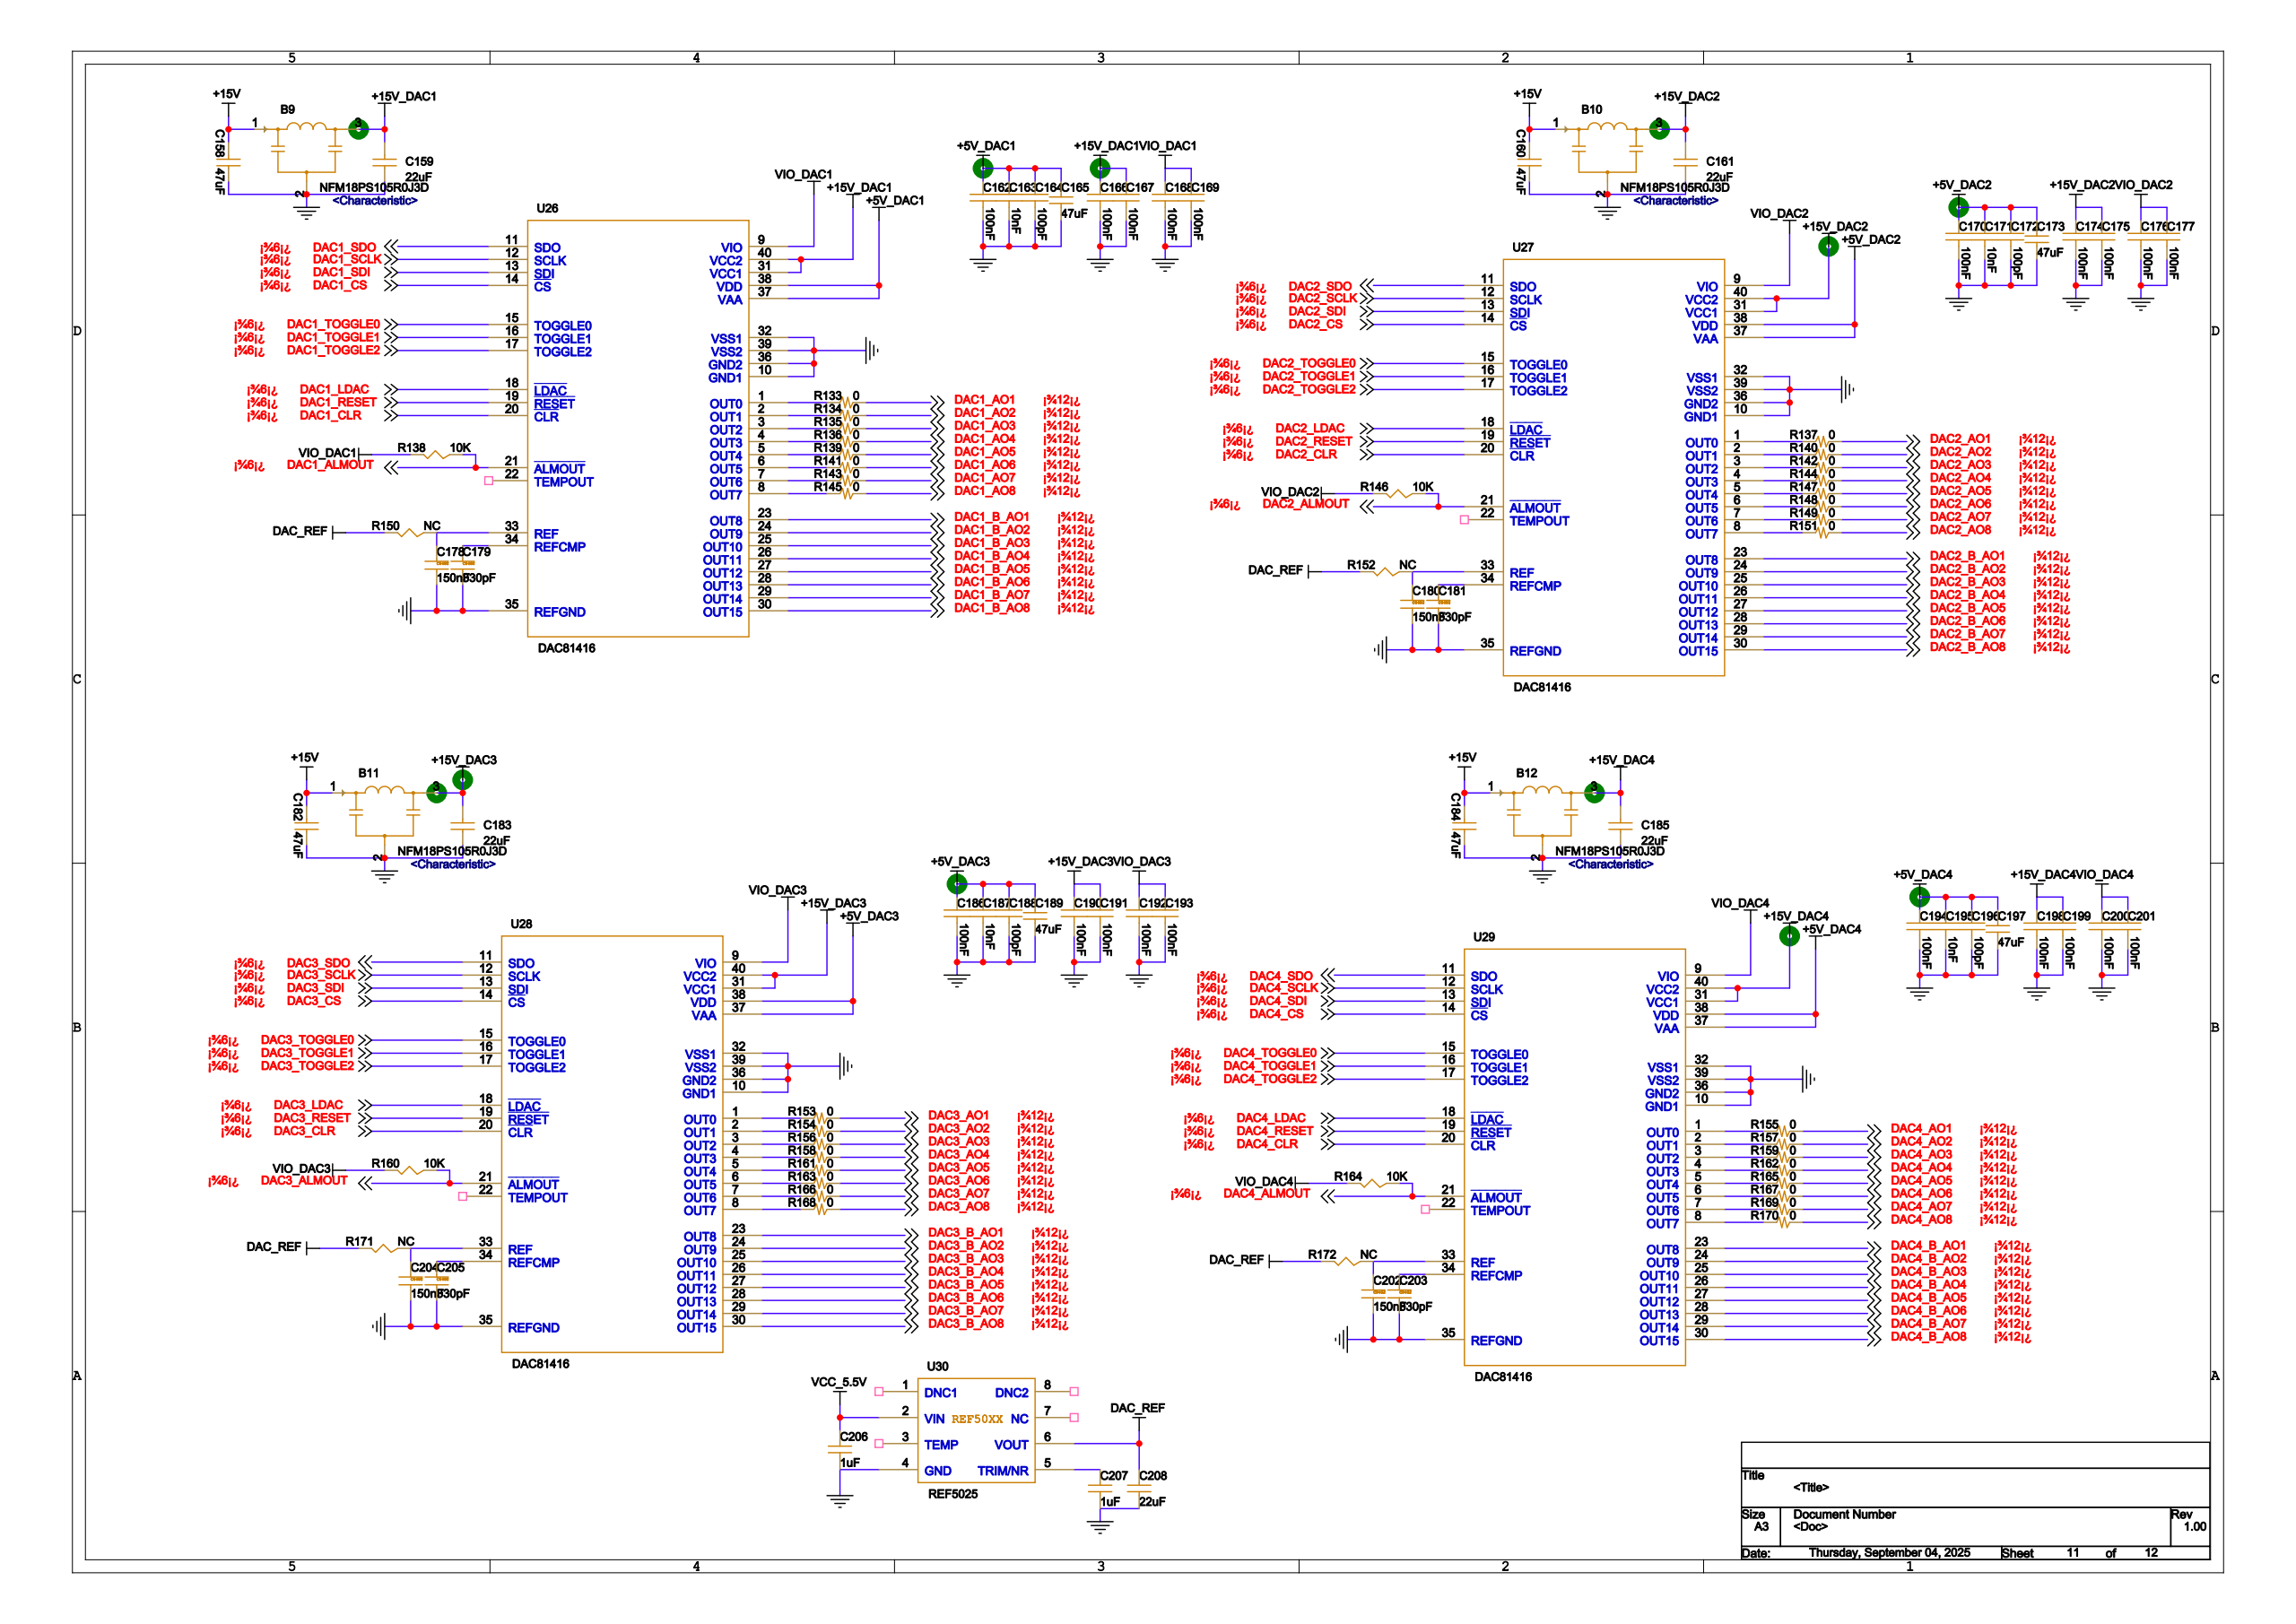Circuit board | Cadence Allegro | 528 parts | 530 nets | one sheet of the schematic
Parts on this sheet (reference | value | footprint):
B9 | NFM18PS105R0J3D | B0603
B10 | NFM18PS105R0J3D | B0603
B11 | NFM18PS105R0J3D | B0603
B12 | NFM18PS105R0J3D | B0603
C158 | 47uF | C0603
C159 | 22uF | C0603
C160 | 47uF | C0603
C161 | 22uF | C0603
C162 | 100nF | C0402
C163 | 10nF | C0402
C164 | 100pF | C0402
C165 | 47uF | C0603
C166 | 100nF | C0402
C167 | 100nF | C0402
C168 | 100nF | C0402
C169 | 100nF | C0402
C170 | 100nF | C0402
C171 | 10nF | C0402
C172 | 100pF | C0402
C173 | 47uF | C0603
C174 | 100nF | C0402
C175 | 100nF | C0402
C176 | 100nF | C0402
C177 | 100nF | C0402
C178 | 150nF | C0402
C179 | 330pF | C0402
C180 | 150nF | C0402
C181 | 330pF | C0402
C182 | 47uF | C0603
C183 | 22uF | C0603
C184 | 47uF | C0603
C185 | 22uF | C0603
C186 | 100nF | C0402
C187 | 10nF | C0402
C188 | 100pF | C0402
C189 | 47uF | C0603
C190 | 100nF | C0402
C191 | 100nF | C0402
C192 | 100nF | C0402
C193 | 100nF | C0402
C194 | 100nF | C0402
C195 | 10nF | C0402
C196 | 100pF | C0402
C197 | 47uF | C0603
C198 | 100nF | C0402
C199 | 100nF | C0402
C200 | 100nF | C0402
C201 | 100nF | C0402
C202 | 150nF | C0402
C203 | 330pF | C0402
C204 | 150nF | C0402
C205 | 330pF | C0402
C206 | 1uF | C0402
C207 | 1uF | C0402
C208 | 22uF | C0603
R133 | 0 | R0402
R134 | 0 | R0402
R135 | 0 | R0402
R136 | 0 | R0402
R137 | 0 | R0402
R138 | 10K | R0402
R139 | 0 | R0402
R140 | 0 | R0402
R141 | 0 | R0402
R142 | 0 | R0402
R143 | 0 | R0402
R144 | 0 | R0402
R145 | 0 | R0402
R146 | 10K | R0402
R147 | 0 | R0402
R148 | 0 | R0402
R149 | 0 | R0402
R150 | NC | R0402
R151 | 0 | R0402
R152 | NC | R0402
R153 | 0 | R0402
R154 | 0 | R0402
R155 | 0 | R0402
R156 | 0 | R0402
R157 | 0 | R0402
R158 | 0 | R0402
R159 | 0 | R0402
R160 | 10K | R0402
R161 | 0 | R0402
R162 | 0 | R0402
R163 | 0 | R0402
R164 | 10K | R0402
R165 | 0 | R0402
R166 | 0 | R0402
R167 | 0 | R0402
R168 | 0 | R0402
R169 | 0 | R0402
R170 | 0 | R0402
R171 | NC | R0402
R172 | NC | R0402
U26 | DAC81416 | VQFN-40
U27 | DAC81416 | VQFN-40
U28 | DAC81416 | VQFN-40
U29 | DAC81416 | VQFN-40
U30 | REF5025 | SOIC-8
Nets of these parts (net: part-pin ...):
+15V: B9-1 B10-1 B11-1 B12-1 C158-2 C160-2 C182-2 C184-2
GND: B9-2 B10-2 B11-2 B12-2 C158-1 C159-1 C160-1 C161-1 C162-2 C163-2 C164-2 C165-2 C166-2 C167-2 C168-2 C169-2 C170-2 C171-2 C172-2 C173-2 C174-2 C175-2 C176-2 C177-2 C178-2 C179-2 C180-2 C181-2 C182-1 C183-1 C184-1 C185-1 C186-2 C187-2 C188-2 C189-2 C190-2 C191-2 C192-2 C193-2 C194-2 C195-2 C196-2 C197-2 C198-2 C199-2 C200-2 C201-2 C202-2 C203-2 C204-2 C205-2 C206-2 C207-2 C208-2 U30-4 U26-10 U26-32 U26-35 U26-36 U26-39 U27-10 U27-32 U27-35 U27-36 U27-39 U28-10 U28-32 U28-35 U28-36 U28-39 U29-10 U29-32 U29-35 U29-36 U29-39
+15V_DAC2: B10-3 C161-2 C174-1 C175-1 U27-31 U27-40
+15V_DAC3: B11-3 C183-2 C190-1 C191-1 U28-31 U28-40
+15V_DAC4: B12-3 C185-2 C198-1 C199-1 U29-31 U29-40
+5V_DAC1: C162-1 C163-1 C164-1 C165-1 U26-37 U26-38
+5V_DAC2: C170-1 C171-1 C172-1 C173-1 U27-37 U27-38
+5V_DAC3: C186-1 C187-1 C188-1 C189-1 U28-37 U28-38
+5V_DAC4: C194-1 C195-1 C196-1 C197-1 U29-37 U29-38
+15V_DAC1: B9-3 C159-2 C166-1 C167-1 U26-31 U26-40
DAC1_B_AO6: U26-28
DAC3_B_AO3: U28-25
DAC1_B_AO5: U26-27
DAC3_B_AO4: U28-26
DAC1_B_AO4: U26-26
DAC3_B_AO5: U28-27
DAC1_B_AO3: U26-25
DAC3_B_AO6: U28-28
DAC1_B_AO2: U26-24
DAC3_B_AO7: U28-29
DAC1_B_AO8: U26-30
DAC1_B_AO1: U26-23
DAC3_B_AO8: U28-30
DAC3_B_AO1: U28-23
DAC1_B_AO7: U26-29
DAC3_B_AO2: U28-24
DAC2_B_AO6: U27-28
DAC4_B_AO3: U29-25
DAC2_B_AO5: U27-27
DAC4_B_AO4: U29-26
DAC2_B_AO4: U27-26
DAC4_B_AO5: U29-27
DAC2_B_AO3: U27-25
DAC4_B_AO6: U29-28
DAC2_B_AO2: U27-24
DAC4_B_AO7: U29-29
DAC2_B_AO8: U27-30
DAC2_B_AO1: U27-23
DAC4_B_AO8: U29-30
DAC4_B_AO1: U29-23
DAC2_B_AO7: U27-29
DAC4_B_AO2: U29-24
VCC_5.5V: C206-1 U30-2
VIO_DAC1: C168-1 C169-1 R138-2 U26-9
VIO_DAC2: C176-1 C177-1 R146-2 U27-9
VIO_DAC3: C192-1 C193-1 R160-2 U28-9
VIO_DAC4: C200-1 C201-1 R164-2 U29-9
DAC_REF: C208-1 R150-2 R152-2 R171-2 R172-2 U30-6
N18747083: C207-1 U30-5
N18725219: C178-1 R150-1 U26-33
N18736758: C180-1 R152-1 U27-33
N18739460: C202-1 R172-1 U29-33
N18738063: C204-1 R171-1 U28-33
N18725228: C179-1 U26-34
N18736769: C181-1 U27-34
N18739471: C203-1 U29-34
N18738074: C205-1 U28-34
DAC3_AO4: R158-2
DAC3_AO3: R156-2
DAC3_AO2: R154-2
DAC3_AO1: R153-2
DAC2_AO8: R151-2
DAC3_AO8: R168-2
DAC2_AO7: R149-2
DAC2_AO6: R148-2
DAC2_AO5: R147-2
DAC2_AO4: R144-2
DAC2_AO3: R142-2
DAC2_AO2: R140-2
DAC2_AO1: R137-2
DAC1_AO1: R133-2
DAC1_AO2: R134-2
DAC3_AO7: R166-2
DAC1_AO3: R135-2
DAC1_AO4: R136-2
DAC1_AO5: R139-2
DAC1_AO6: R141-2
DAC1_AO7: R143-2
DAC1_AO8: R145-2
DAC4_AO1: R155-2
DAC4_AO2: R157-2
DAC4_AO3: R159-2
DAC4_AO4: R162-2
DAC3_AO6: R163-2
DAC4_AO5: R165-2
DAC4_AO6: R167-2
DAC4_AO7: R169-2
DAC4_AO8: R170-2
DAC3_AO5: R161-2
DAC1_ALMOUT: R138-1 U26-21
DAC2_ALMOUT: R146-1 U27-21
DAC3_ALMOUT: R160-1 U28-21
DAC4_ALMOUT: R164-1 U29-21
N18725545: R133-1 U26-1
N18725561: R134-1 U26-2
N18725566: R135-1 U26-3
N18725575: R136-1 U26-4
N18736614: R137-1 U27-1
N18725584: R139-1 U26-5
N18736633: R140-1 U27-2
N18725593: R141-1 U26-6
N18736650: R142-1 U27-3
N18725602: R143-1 U26-7
N18736667: R144-1 U27-4
N18726122: R145-1 U26-8
N18736689: R147-1 U27-5
N18736708: R148-1 U27-6
N18736725: R149-1 U27-7
N18736742: R151-1 U27-8
N18737919: R153-1 U28-1
N18737938: R154-1 U28-2
N18739316: R155-1 U29-1
N18737955: R156-1 U28-3
N18739335: R157-1 U29-2
N18737972: R158-1 U28-4
N18739352: R159-1 U29-3
N18737994: R161-1 U28-5
N18739369: R162-1 U29-4
N18738013: R163-1 U28-6
N18739391: R165-1 U29-5
N18738030: R166-1 U28-7
N18739410: R167-1 U29-6
N18738047: R168-1 U28-8
N18739427: R169-1 U29-7
N18739444: R170-1 U29-8
DAC3_SDO: U28-11
DAC3_SCLK: U28-12
DAC3_SDI: U28-13
DAC3_CS: U28-14
DAC3_TOGGLE0: U28-15
DAC3_TOGGLE1: U28-16
DAC3_TOGGLE2: U28-17
DAC3_LDAC: U28-18
DAC3_RESET: U28-19
DAC3_CLR: U28-20
DAC4_SDO: U29-11
DAC4_SCLK: U29-12
DAC4_SDI: U29-13
DAC4_CS: U29-14
DAC4_TOGGLE1: U29-16
DAC4_TOGGLE2: U29-17
DAC4_TOGGLE0: U29-15
DAC4_LDAC: U29-18
DAC4_RESET: U29-19
DAC4_CLR: U29-20
DAC1_SDO: U26-11
DAC1_SCLK: U26-12
DAC1_SDI: U26-13
DAC1_CS: U26-14
DAC1_TOGGLE0: U26-15
DAC1_TOGGLE1: U26-16
DAC1_TOGGLE2: U26-17
DAC1_LDAC: U26-18
DAC1_RESET: U26-19
DAC1_CLR: U26-20
DAC2_SDO: U27-11
DAC2_SCLK: U27-12
DAC2_SDI: U27-13
DAC2_CS: U27-14
DAC2_TOGGLE1: U27-16
DAC2_TOGGLE2: U27-17
DAC2_TOGGLE0: U27-15
DAC2_LDAC: U27-18
DAC2_RESET: U27-19
DAC2_CLR: U27-20